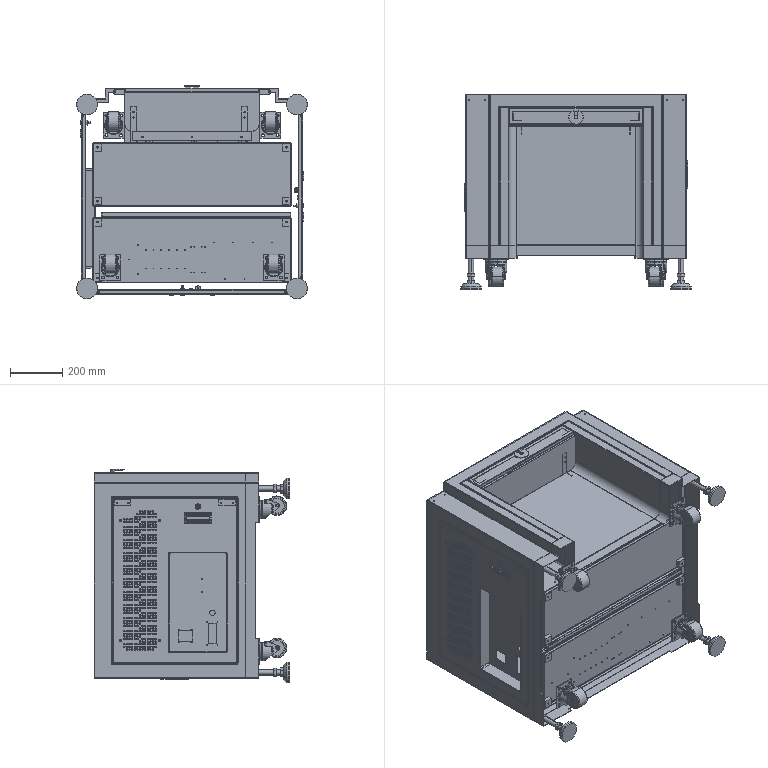Part | SolidWorks | features HoleWzd 1 | 102 solids | 5006 faces | volume 9143617 mm3 | cylinder 2657 | plane 1785 | spline 252 | cone 192 | torus 116 | sphere 4 | commonest cylinder face diameters 5 x1116 3.3 x204 6 x139 1 x98 10 x94 4.5 x80